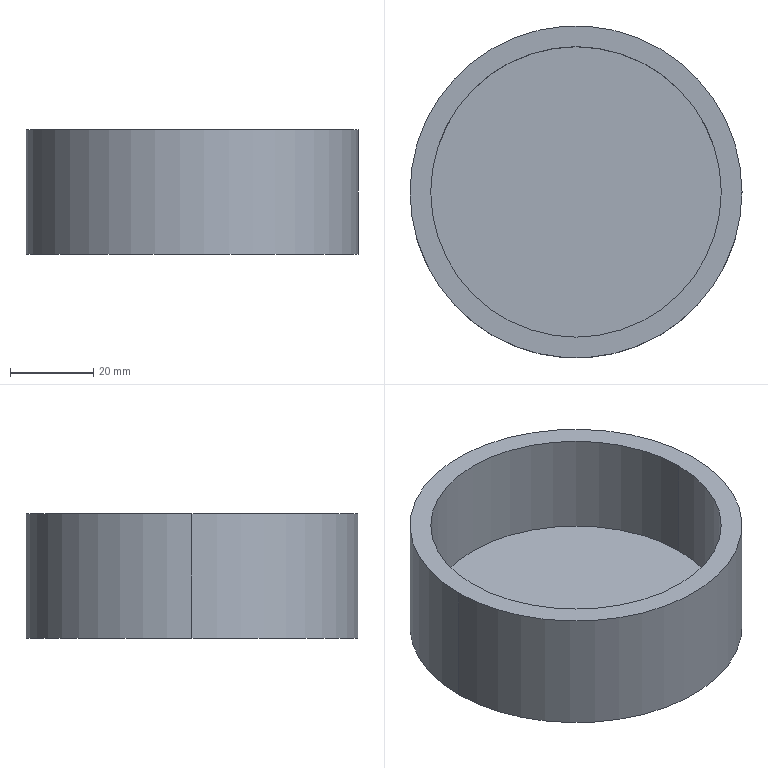Part | SolidWorks | features Extrusion 1, ICE 1 | 1 solid | 7 faces | box 80 x 80 x 30 mm | volume 54585 mm3 | cylinder 4 | plane 3 | commonest cylinder face diameters 70 x2 80 x2
STEP:
#1=CARTESIAN_POINT('',(-35.,0.,30.));
#2=VERTEX_POINT('',#1);
#3=CARTESIAN_POINT('',(35.,0.,30.));
#4=VERTEX_POINT('',#3);
#5=CARTESIAN_POINT('',(0.,0.,30.));
#6=DIRECTION('',(0.,0.,1.));
#7=DIRECTION('',(1.,0.,0.));
#8=AXIS2_PLACEMENT_3D('',#5,#6,#7);
#9=CIRCLE('',#8,35.);
#10=EDGE_CURVE('',#2,#4,#9,.T.);
#11=ORIENTED_EDGE('',*,*,#10,.T.);
#12=CARTESIAN_POINT('',(35.,0.,5.));
#13=VERTEX_POINT('',#12);
#14=CARTESIAN_POINT('',(35.,0.,30.));
#15=DIRECTION('',(0.,0.,-1.));
#16=VECTOR('',#15,1000.);
#17=LINE('',#14,#16);
#18=EDGE_CURVE('',#4,#13,#17,.T.);
#19=ORIENTED_EDGE('',*,*,#18,.T.);
#20=CARTESIAN_POINT('',(-35.,0.,5.));
#21=VERTEX_POINT('',#20);
#22=CARTESIAN_POINT('',(0.,0.,5.));
#23=DIRECTION('',(0.,0.,-1.));
#24=DIRECTION('',(1.,0.,0.));
#25=AXIS2_PLACEMENT_3D('',#22,#23,#24);
#26=CIRCLE('',#25,35.);
#27=EDGE_CURVE('',#13,#21,#26,.T.);
#28=ORIENTED_EDGE('',*,*,#27,.T.);
#29=CARTESIAN_POINT('',(-35.,0.,30.));
#30=DIRECTION('',(0.,0.,-1.));
#31=VECTOR('',#30,1000.);
#32=LINE('',#29,#31);
#33=EDGE_CURVE('',#2,#21,#32,.T.);
#34=ORIENTED_EDGE('',*,*,#33,.F.);
#35=EDGE_LOOP('',(#11,#19,#28,#34));
#36=FACE_OUTER_BOUND('',#35,.T.);
#37=CARTESIAN_POINT('',(0.,0.,30.));
#38=DIRECTION('',(0.,0.,-1.));
#39=DIRECTION('',(-1.,0.,0.));
#40=AXIS2_PLACEMENT_3D('',#37,#38,#39);
#41=CYLINDRICAL_SURFACE('',#40,35.);
#42=ADVANCED_FACE('',(#36),#41,.F.);
#43=CARTESIAN_POINT('',(40.,0.,30.));
#44=VERTEX_POINT('',#43);
#45=CARTESIAN_POINT('',(-40.,0.,30.));
#46=VERTEX_POINT('',#45);
#47=CARTESIAN_POINT('',(0.,0.,30.));
#48=DIRECTION('',(0.,0.,1.));
#49=DIRECTION('',(1.,0.,0.));
#50=AXIS2_PLACEMENT_3D('',#47,#48,#49);
#51=CIRCLE('',#50,40.);
#52=EDGE_CURVE('',#44,#46,#51,.T.);
#53=ORIENTED_EDGE('',*,*,#52,.F.);
#54=CARTESIAN_POINT('',(40.,0.,0.));
#55=VERTEX_POINT('',#54);
#56=CARTESIAN_POINT('',(40.,0.,5.));
#57=DIRECTION('',(0.,0.,-1.));
#58=VECTOR('',#57,1000.);
#59=LINE('',#56,#58);
#60=EDGE_CURVE('',#44,#55,#59,.T.);
#61=ORIENTED_EDGE('',*,*,#60,.T.);
#62=CARTESIAN_POINT('',(-40.,0.,0.));
#63=VERTEX_POINT('',#62);
#64=CARTESIAN_POINT('',(0.,0.,0.));
#65=DIRECTION('',(0.,0.,1.));
#66=DIRECTION('',(1.,0.,0.));
#67=AXIS2_PLACEMENT_3D('',#64,#65,#66);
#68=CIRCLE('',#67,40.);
#69=EDGE_CURVE('',#55,#63,#68,.T.);
#70=ORIENTED_EDGE('',*,*,#69,.T.);
#71=CARTESIAN_POINT('',(-40.,0.,5.));
#72=DIRECTION('',(0.,0.,-1.));
#73=VECTOR('',#72,1000.);
#74=LINE('',#71,#73);
#75=EDGE_CURVE('',#46,#63,#74,.T.);
#76=ORIENTED_EDGE('',*,*,#75,.F.);
#77=EDGE_LOOP('',(#53,#61,#70,#76));
#78=FACE_OUTER_BOUND('',#77,.T.);
#79=CARTESIAN_POINT('',(0.,0.,5.));
#80=DIRECTION('',(0.,0.,-1.));
#81=DIRECTION('',(-1.,0.,0.));
#82=AXIS2_PLACEMENT_3D('',#79,#80,#81);
#83=CYLINDRICAL_SURFACE('',#82,40.);
#84=ADVANCED_FACE('',(#78),#83,.T.);
#85=ORIENTED_EDGE('',*,*,#60,.F.);
#86=CARTESIAN_POINT('',(0.,0.,30.));
#87=DIRECTION('',(0.,0.,1.));
#88=DIRECTION('',(1.,0.,0.));
#89=AXIS2_PLACEMENT_3D('',#86,#87,#88);
#90=CIRCLE('',#89,40.);
#91=EDGE_CURVE('',#46,#44,#90,.T.);
#92=ORIENTED_EDGE('',*,*,#91,.F.);
#93=ORIENTED_EDGE('',*,*,#75,.T.);
#94=CARTESIAN_POINT('',(0.,0.,0.));
#95=DIRECTION('',(0.,0.,1.));
#96=DIRECTION('',(1.,0.,0.));
#97=AXIS2_PLACEMENT_3D('',#94,#95,#96);
#98=CIRCLE('',#97,40.);
#99=EDGE_CURVE('',#63,#55,#98,.T.);
#100=ORIENTED_EDGE('',*,*,#99,.T.);
#101=EDGE_LOOP('',(#85,#92,#93,#100));
#102=FACE_OUTER_BOUND('',#101,.T.);
#103=CARTESIAN_POINT('',(0.,0.,5.));
#104=DIRECTION('',(0.,0.,-1.));
#105=DIRECTION('',(-1.,0.,0.));
#106=AXIS2_PLACEMENT_3D('',#103,#104,#105);
#107=CYLINDRICAL_SURFACE('',#106,40.);
#108=ADVANCED_FACE('',(#102),#107,.T.);
#109=ORIENTED_EDGE('',*,*,#99,.F.);
#110=ORIENTED_EDGE('',*,*,#69,.F.);
#111=EDGE_LOOP('',(#109,#110));
#112=FACE_OUTER_BOUND('',#111,.T.);
#113=CARTESIAN_POINT('',(0.,0.,0.));
#114=DIRECTION('',(0.,0.,1.));
#115=DIRECTION('',(1.,0.,0.));
#116=AXIS2_PLACEMENT_3D('',#113,#114,#115);
#117=PLANE('',#116);
#118=ADVANCED_FACE('',(#112),#117,.F.);
#119=ORIENTED_EDGE('',*,*,#91,.T.);
#120=ORIENTED_EDGE('',*,*,#52,.T.);
#121=EDGE_LOOP('',(#119,#120));
#122=FACE_OUTER_BOUND('',#121,.T.);
#123=ORIENTED_EDGE('',*,*,#10,.F.);
#124=CARTESIAN_POINT('',(0.,0.,30.));
#125=DIRECTION('',(0.,0.,1.));
#126=DIRECTION('',(1.,0.,0.));
#127=AXIS2_PLACEMENT_3D('',#124,#125,#126);
#128=CIRCLE('',#127,35.);
#129=EDGE_CURVE('',#4,#2,#128,.T.);
#130=ORIENTED_EDGE('',*,*,#129,.F.);
#131=EDGE_LOOP('',(#123,#130));
#132=FACE_BOUND('',#131,.T.);
#133=CARTESIAN_POINT('',(0.,0.,30.));
#134=DIRECTION('',(0.,0.,1.));
#135=DIRECTION('',(1.,0.,0.));
#136=AXIS2_PLACEMENT_3D('',#133,#134,#135);
#137=PLANE('',#136);
#138=ADVANCED_FACE('',(#122,#132),#137,.T.);
#139=ORIENTED_EDGE('',*,*,#18,.F.);
#140=ORIENTED_EDGE('',*,*,#129,.T.);
#141=ORIENTED_EDGE('',*,*,#33,.T.);
#142=CARTESIAN_POINT('',(0.,0.,5.));
#143=DIRECTION('',(0.,0.,-1.));
#144=DIRECTION('',(1.,0.,0.));
#145=AXIS2_PLACEMENT_3D('',#142,#143,#144);
#146=CIRCLE('',#145,35.);
#147=EDGE_CURVE('',#21,#13,#146,.T.);
#148=ORIENTED_EDGE('',*,*,#147,.T.);
#149=EDGE_LOOP('',(#139,#140,#141,#148));
#150=FACE_OUTER_BOUND('',#149,.T.);
#151=CARTESIAN_POINT('',(0.,0.,30.));
#152=DIRECTION('',(0.,0.,-1.));
#153=DIRECTION('',(-1.,0.,0.));
#154=AXIS2_PLACEMENT_3D('',#151,#152,#153);
#155=CYLINDRICAL_SURFACE('',#154,35.);
#156=ADVANCED_FACE('',(#150),#155,.F.);
#157=ORIENTED_EDGE('',*,*,#147,.F.);
#158=ORIENTED_EDGE('',*,*,#27,.F.);
#159=EDGE_LOOP('',(#157,#158));
#160=FACE_OUTER_BOUND('',#159,.T.);
#161=CARTESIAN_POINT('',(0.,0.,5.));
#162=DIRECTION('',(0.,0.,1.));
#163=DIRECTION('',(1.,0.,0.));
#164=AXIS2_PLACEMENT_3D('',#161,#162,#163);
#165=PLANE('',#164);
#166=ADVANCED_FACE('',(#160),#165,.T.);
#167=CLOSED_SHELL('',(#42,#84,#108,#118,#138,#156,#166));
#168=MANIFOLD_SOLID_BREP('',#167);
#169=CARTESIAN_POINT('',(0.,0.,0.));
#170=DIRECTION('',(0.,0.,1.));
#171=DIRECTION('',(1.,0.,0.));
#172=AXIS2_PLACEMENT_3D('',#169,#170,#171);
#173=(LENGTH_UNIT()NAMED_UNIT(*)SI_UNIT(.MILLI.,.METRE.));
#174=UNCERTAINTY_MEASURE_WITH_UNIT(LENGTH_MEASURE(0.00001),#173,'','');
#175=(NAMED_UNIT(*)PLANE_ANGLE_UNIT()SI_UNIT($,.RADIAN.));
#176=(NAMED_UNIT(*)SI_UNIT($,.STERADIAN.)SOLID_ANGLE_UNIT());
#177=(GEOMETRIC_REPRESENTATION_CONTEXT(3)GLOBAL_UNCERTAINTY_ASSIGNED_CONTEXT((#174))GLOBAL_UNIT_ASSIGNED_CONTEXT((#173,#175,#176))REPRESENTATION_CONTEXT('',''));
#178=ADVANCED_BREP_SHAPE_REPRESENTATION('',(#168,#172),#177);